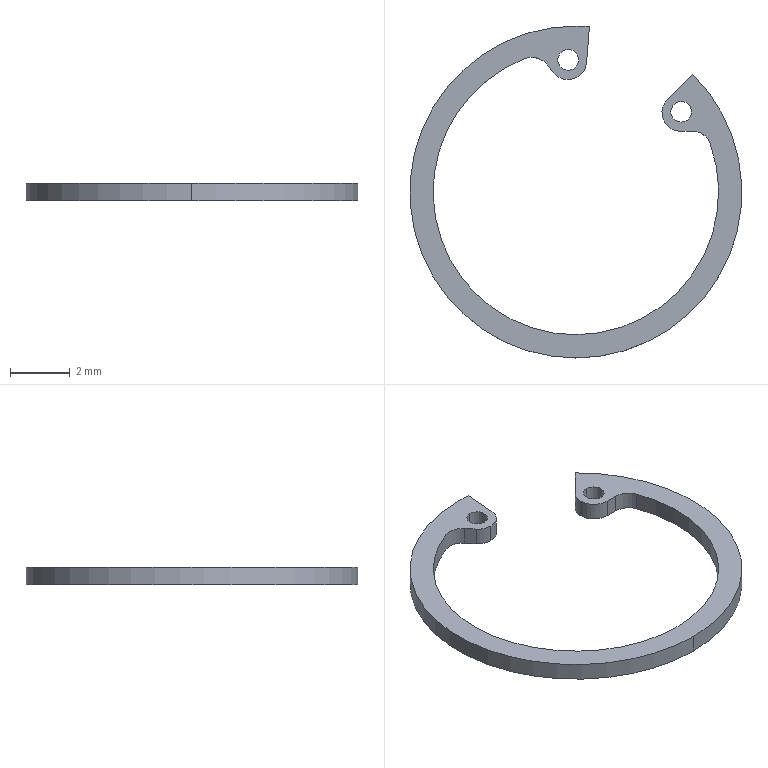Part | SolidWorks | features BaseBody 1 | 1 solid | 21 faces | box 11.1 x 11.1 x 0.6 mm | volume 14.442 mm3 | cylinder 15 | plane 6 | commonest cylinder face diameters 1.243 x6 0.694 x4 11.1 x3 9.546 x2
STEP:
#1=CARTESIAN_POINT('',(558.117,-169.855,283.191));
#2=VERTEX_POINT('',#1);
#3=CARTESIAN_POINT('',(558.117,-169.161,283.191));
#4=VERTEX_POINT('',#3);
#5=CARTESIAN_POINT('',(558.117,-169.508,283.191));
#6=DIRECTION('',(-0.000000001,0.000000003,-1.));
#7=DIRECTION('',(0.,1.,0.000000003));
#8=AXIS2_PLACEMENT_3D('',#5,#6,#7);
#9=CIRCLE('',#8,0.3469);
#10=EDGE_CURVE('',#2,#4,#9,.T.);
#11=ORIENTED_EDGE('',*,*,#10,.F.);
#12=CARTESIAN_POINT('',(558.117,-169.855,282.591));
#13=VERTEX_POINT('',#12);
#14=CARTESIAN_POINT('',(558.117,-169.855,282.591));
#15=DIRECTION('',(-0.000000001,0.000000003,-1.));
#16=VECTOR('',#15,1000.);
#17=LINE('',#14,#16);
#18=EDGE_CURVE('',#2,#13,#17,.T.);
#19=ORIENTED_EDGE('',*,*,#18,.T.);
#20=CARTESIAN_POINT('',(558.117,-169.161,282.591));
#21=VERTEX_POINT('',#20);
#22=CARTESIAN_POINT('',(558.117,-169.508,282.591));
#23=DIRECTION('',(0.000000001,-0.000000003,1.));
#24=DIRECTION('',(0.,1.,0.000000003));
#25=AXIS2_PLACEMENT_3D('',#22,#23,#24);
#26=CIRCLE('',#25,0.3469);
#27=EDGE_CURVE('',#21,#13,#26,.T.);
#28=ORIENTED_EDGE('',*,*,#27,.F.);
#29=CARTESIAN_POINT('',(558.117,-169.161,282.591));
#30=DIRECTION('',(-0.000000001,0.000000003,-1.));
#31=VECTOR('',#30,1000.);
#32=LINE('',#29,#31);
#33=EDGE_CURVE('',#4,#21,#32,.T.);
#34=ORIENTED_EDGE('',*,*,#33,.F.);
#35=EDGE_LOOP('',(#11,#19,#28,#34));
#36=FACE_OUTER_BOUND('',#35,.T.);
#37=CARTESIAN_POINT('',(558.117,-169.508,282.591));
#38=DIRECTION('',(-0.000000001,0.000000003,-1.));
#39=DIRECTION('',(0.,1.,0.000000003));
#40=AXIS2_PLACEMENT_3D('',#37,#38,#39);
#41=CYLINDRICAL_SURFACE('',#40,0.3469);
#42=ADVANCED_FACE('',(#36),#41,.F.);
#43=CARTESIAN_POINT('',(561.892,-171.592,283.191));
#44=VERTEX_POINT('',#43);
#45=CARTESIAN_POINT('',(561.892,-170.898,283.191));
#46=VERTEX_POINT('',#45);
#47=CARTESIAN_POINT('',(561.892,-171.245,283.191));
#48=DIRECTION('',(-0.000000001,0.000000003,-1.));
#49=DIRECTION('',(0.,1.,0.000000003));
#50=AXIS2_PLACEMENT_3D('',#47,#48,#49);
#51=CIRCLE('',#50,0.3469);
#52=EDGE_CURVE('',#44,#46,#51,.T.);
#53=ORIENTED_EDGE('',*,*,#52,.F.);
#54=CARTESIAN_POINT('',(561.892,-171.592,282.591));
#55=VERTEX_POINT('',#54);
#56=CARTESIAN_POINT('',(561.892,-171.592,282.591));
#57=DIRECTION('',(-0.000000001,0.000000003,-1.));
#58=VECTOR('',#57,1000.);
#59=LINE('',#56,#58);
#60=EDGE_CURVE('',#44,#55,#59,.T.);
#61=ORIENTED_EDGE('',*,*,#60,.T.);
#62=CARTESIAN_POINT('',(561.892,-170.898,282.591));
#63=VERTEX_POINT('',#62);
#64=CARTESIAN_POINT('',(561.892,-171.245,282.591));
#65=DIRECTION('',(0.000000001,-0.000000003,1.));
#66=DIRECTION('',(0.,1.,0.000000003));
#67=AXIS2_PLACEMENT_3D('',#64,#65,#66);
#68=CIRCLE('',#67,0.3469);
#69=EDGE_CURVE('',#63,#55,#68,.T.);
#70=ORIENTED_EDGE('',*,*,#69,.F.);
#71=CARTESIAN_POINT('',(561.892,-170.898,282.591));
#72=DIRECTION('',(-0.000000001,0.000000003,-1.));
#73=VECTOR('',#72,1000.);
#74=LINE('',#71,#73);
#75=EDGE_CURVE('',#46,#63,#74,.T.);
#76=ORIENTED_EDGE('',*,*,#75,.F.);
#77=EDGE_LOOP('',(#53,#61,#70,#76));
#78=FACE_OUTER_BOUND('',#77,.T.);
#79=CARTESIAN_POINT('',(561.892,-171.245,282.591));
#80=DIRECTION('',(-0.000000001,0.000000003,-1.));
#81=DIRECTION('',(0.,1.,0.000000003));
#82=AXIS2_PLACEMENT_3D('',#79,#80,#81);
#83=CYLINDRICAL_SURFACE('',#82,0.3469);
#84=ADVANCED_FACE('',(#78),#83,.F.);
#85=CARTESIAN_POINT('',(561.428,-170.838,282.591));
#86=VERTEX_POINT('',#85);
#87=CARTESIAN_POINT('',(561.87,-171.897,282.591));
#88=VERTEX_POINT('',#87);
#89=CARTESIAN_POINT('',(561.87,-171.275,282.591));
#90=DIRECTION('',(0.000000001,-0.000000003,1.));
#91=DIRECTION('',(0.,-1.,-0.000000003));
#92=AXIS2_PLACEMENT_3D('',#89,#90,#91);
#93=CIRCLE('',#92,0.6216);
#94=EDGE_CURVE('',#86,#88,#93,.T.);
#95=ORIENTED_EDGE('',*,*,#94,.T.);
#96=CARTESIAN_POINT('',(561.87,-171.897,283.191));
#97=VERTEX_POINT('',#96);
#98=CARTESIAN_POINT('',(561.87,-171.897,282.591));
#99=DIRECTION('',(0.000000001,-0.000000003,1.));
#100=VECTOR('',#99,1000.);
#101=LINE('',#98,#100);
#102=EDGE_CURVE('',#88,#97,#101,.T.);
#103=ORIENTED_EDGE('',*,*,#102,.T.);
#104=CARTESIAN_POINT('',(561.428,-170.838,283.191));
#105=VERTEX_POINT('',#104);
#106=CARTESIAN_POINT('',(561.87,-171.275,283.191));
#107=DIRECTION('',(0.000000001,-0.000000003,1.));
#108=DIRECTION('',(0.,-1.,-0.000000003));
#109=AXIS2_PLACEMENT_3D('',#106,#107,#108);
#110=CIRCLE('',#109,0.6216);
#111=EDGE_CURVE('',#105,#97,#110,.T.);
#112=ORIENTED_EDGE('',*,*,#111,.F.);
#113=CARTESIAN_POINT('',(561.428,-170.838,282.591));
#114=DIRECTION('',(-0.000000001,0.000000003,-1.));
#115=VECTOR('',#114,1000.);
#116=LINE('',#113,#115);
#117=EDGE_CURVE('',#105,#86,#116,.T.);
#118=ORIENTED_EDGE('',*,*,#117,.T.);
#119=EDGE_LOOP('',(#95,#103,#112,#118));
#120=FACE_OUTER_BOUND('',#119,.T.);
#121=CARTESIAN_POINT('',(561.87,-171.275,282.591));
#122=DIRECTION('',(0.000000001,-0.000000003,1.));
#123=DIRECTION('',(0.,-1.,-0.000000003));
#124=AXIS2_PLACEMENT_3D('',#121,#122,#123);
#125=CYLINDRICAL_SURFACE('',#124,0.6216);
#126=ADVANCED_FACE('',(#120),#125,.T.);
#127=CARTESIAN_POINT('',(558.826,-168.395,282.591));
#128=VERTEX_POINT('',#127);
#129=CARTESIAN_POINT('',(558.371,-168.377,282.591));
#130=VERTEX_POINT('',#129);
#131=CARTESIAN_POINT('',(558.371,-173.927,282.591));
#132=DIRECTION('',(0.000000001,-0.000000003,1.));
#133=DIRECTION('',(0.,-1.,-0.000000003));
#134=AXIS2_PLACEMENT_3D('',#131,#132,#133);
#135=CIRCLE('',#134,5.55);
#136=EDGE_CURVE('',#128,#130,#135,.T.);
#137=ORIENTED_EDGE('',*,*,#136,.T.);
#138=CARTESIAN_POINT('',(558.371,-168.377,283.191));
#139=VERTEX_POINT('',#138);
#140=CARTESIAN_POINT('',(558.371,-168.377,282.591));
#141=DIRECTION('',(0.000000001,-0.000000003,1.));
#142=VECTOR('',#141,1000.);
#143=LINE('',#140,#142);
#144=EDGE_CURVE('',#130,#139,#143,.T.);
#145=ORIENTED_EDGE('',*,*,#144,.T.);
#146=CARTESIAN_POINT('',(558.826,-168.395,283.191));
#147=VERTEX_POINT('',#146);
#148=CARTESIAN_POINT('',(558.371,-173.927,283.191));
#149=DIRECTION('',(0.000000001,-0.000000003,1.));
#150=DIRECTION('',(0.,-1.,-0.000000003));
#151=AXIS2_PLACEMENT_3D('',#148,#149,#150);
#152=CIRCLE('',#151,5.55);
#153=EDGE_CURVE('',#147,#139,#152,.T.);
#154=ORIENTED_EDGE('',*,*,#153,.F.);
#155=CARTESIAN_POINT('',(558.826,-168.395,282.591));
#156=DIRECTION('',(-0.000000001,0.000000003,-1.));
#157=VECTOR('',#156,1000.);
#158=LINE('',#155,#157);
#159=EDGE_CURVE('',#147,#128,#158,.T.);
#160=ORIENTED_EDGE('',*,*,#159,.T.);
#161=EDGE_LOOP('',(#137,#145,#154,#160));
#162=FACE_OUTER_BOUND('',#161,.T.);
#163=CARTESIAN_POINT('',(558.371,-173.927,282.591));
#164=DIRECTION('',(0.000000001,-0.000000003,1.));
#165=DIRECTION('',(0.,-1.,-0.000000003));
#166=AXIS2_PLACEMENT_3D('',#163,#164,#165);
#167=CYLINDRICAL_SURFACE('',#166,5.55);
#168=ADVANCED_FACE('',(#162),#167,.T.);
#169=ORIENTED_EDGE('',*,*,#144,.F.);
#170=CARTESIAN_POINT('',(558.371,-179.477,282.591));
#171=VERTEX_POINT('',#170);
#172=CARTESIAN_POINT('',(558.371,-173.927,282.591));
#173=DIRECTION('',(0.000000001,-0.000000003,1.));
#174=DIRECTION('',(0.,-1.,-0.000000003));
#175=AXIS2_PLACEMENT_3D('',#172,#173,#174);
#176=CIRCLE('',#175,5.55);
#177=EDGE_CURVE('',#130,#171,#176,.T.);
#178=ORIENTED_EDGE('',*,*,#177,.T.);
#179=CARTESIAN_POINT('',(558.371,-179.477,283.191));
#180=VERTEX_POINT('',#179);
#181=CARTESIAN_POINT('',(558.371,-179.477,282.591));
#182=DIRECTION('',(0.000000001,-0.000000003,1.));
#183=VECTOR('',#182,1000.);
#184=LINE('',#181,#183);
#185=EDGE_CURVE('',#171,#180,#184,.T.);
#186=ORIENTED_EDGE('',*,*,#185,.T.);
#187=CARTESIAN_POINT('',(558.371,-173.927,283.191));
#188=DIRECTION('',(0.000000001,-0.000000003,1.));
#189=DIRECTION('',(0.,-1.,-0.000000003));
#190=AXIS2_PLACEMENT_3D('',#187,#188,#189);
#191=CIRCLE('',#190,5.55);
#192=EDGE_CURVE('',#139,#180,#191,.T.);
#193=ORIENTED_EDGE('',*,*,#192,.F.);
#194=EDGE_LOOP('',(#169,#178,#186,#193));
#195=FACE_OUTER_BOUND('',#194,.T.);
#196=CARTESIAN_POINT('',(558.371,-173.927,282.591));
#197=DIRECTION('',(0.000000001,-0.000000003,1.));
#198=DIRECTION('',(0.,-1.,-0.000000003));
#199=AXIS2_PLACEMENT_3D('',#196,#197,#198);
#200=CYLINDRICAL_SURFACE('',#199,5.55);
#201=ADVANCED_FACE('',(#195),#200,.T.);
#202=CARTESIAN_POINT('',(557.631,-169.943,282.591));
#203=VERTEX_POINT('',#202);
#204=CARTESIAN_POINT('',(558.108,-170.166,282.591));
#205=VERTEX_POINT('',#204);
#206=CARTESIAN_POINT('',(558.108,-169.545,282.591));
#207=DIRECTION('',(0.000000001,-0.000000003,1.));
#208=DIRECTION('',(0.,-1.,-0.000000003));
#209=AXIS2_PLACEMENT_3D('',#206,#207,#208);
#210=CIRCLE('',#209,0.6216);
#211=EDGE_CURVE('',#203,#205,#210,.T.);
#212=ORIENTED_EDGE('',*,*,#211,.T.);
#213=CARTESIAN_POINT('',(558.108,-170.166,283.191));
#214=VERTEX_POINT('',#213);
#215=CARTESIAN_POINT('',(558.108,-170.166,282.591));
#216=DIRECTION('',(0.000000001,-0.000000003,1.));
#217=VECTOR('',#216,1000.);
#218=LINE('',#215,#217);
#219=EDGE_CURVE('',#205,#214,#218,.T.);
#220=ORIENTED_EDGE('',*,*,#219,.T.);
#221=CARTESIAN_POINT('',(557.631,-169.943,283.191));
#222=VERTEX_POINT('',#221);
#223=CARTESIAN_POINT('',(558.108,-169.545,283.191));
#224=DIRECTION('',(0.000000001,-0.000000003,1.));
#225=DIRECTION('',(0.,-1.,-0.000000003));
#226=AXIS2_PLACEMENT_3D('',#223,#224,#225);
#227=CIRCLE('',#226,0.6216);
#228=EDGE_CURVE('',#222,#214,#227,.T.);
#229=ORIENTED_EDGE('',*,*,#228,.F.);
#230=CARTESIAN_POINT('',(557.631,-169.943,282.591));
#231=DIRECTION('',(-0.000000001,0.000000003,-1.));
#232=VECTOR('',#231,1000.);
#233=LINE('',#230,#232);
#234=EDGE_CURVE('',#222,#203,#233,.T.);
#235=ORIENTED_EDGE('',*,*,#234,.T.);
#236=EDGE_LOOP('',(#212,#220,#229,#235));
#237=FACE_OUTER_BOUND('',#236,.T.);
#238=CARTESIAN_POINT('',(558.108,-169.545,282.591));
#239=DIRECTION('',(0.000000001,-0.000000003,1.));
#240=DIRECTION('',(0.,-1.,-0.000000003));
#241=AXIS2_PLACEMENT_3D('',#238,#239,#240);
#242=CYLINDRICAL_SURFACE('',#241,0.6216);
#243=ADVANCED_FACE('',(#237),#242,.T.);
#244=CARTESIAN_POINT('',(558.371,-178.7,282.591));
#245=VERTEX_POINT('',#244);
#246=CARTESIAN_POINT('',(562.859,-172.302,282.591));
#247=VERTEX_POINT('',#246);
#248=CARTESIAN_POINT('',(558.371,-173.927,282.591));
#249=DIRECTION('',(0.000000001,-0.000000003,1.));
#250=DIRECTION('',(0.,-1.,-0.000000003));
#251=AXIS2_PLACEMENT_3D('',#248,#249,#250);
#252=CIRCLE('',#251,4.773);
#253=EDGE_CURVE('',#245,#247,#252,.T.);
#254=ORIENTED_EDGE('',*,*,#253,.F.);
#255=CARTESIAN_POINT('',(558.371,-178.7,283.191));
#256=VERTEX_POINT('',#255);
#257=CARTESIAN_POINT('',(558.371,-178.7,282.591));
#258=DIRECTION('',(0.000000001,-0.000000003,1.));
#259=VECTOR('',#258,1000.);
#260=LINE('',#257,#259);
#261=EDGE_CURVE('',#245,#256,#260,.T.);
#262=ORIENTED_EDGE('',*,*,#261,.T.);
#263=CARTESIAN_POINT('',(562.859,-172.302,283.191));
#264=VERTEX_POINT('',#263);
#265=CARTESIAN_POINT('',(558.371,-173.927,283.191));
#266=DIRECTION('',(-0.000000001,0.000000003,-1.));
#267=DIRECTION('',(0.,-1.,-0.000000003));
#268=AXIS2_PLACEMENT_3D('',#265,#266,#267);
#269=CIRCLE('',#268,4.773);
#270=EDGE_CURVE('',#264,#256,#269,.T.);
#271=ORIENTED_EDGE('',*,*,#270,.F.);
#272=CARTESIAN_POINT('',(562.859,-172.302,282.591));
#273=DIRECTION('',(0.000000001,-0.000000003,1.));
#274=VECTOR('',#273,1000.);
#275=LINE('',#272,#274);
#276=EDGE_CURVE('',#247,#264,#275,.T.);
#277=ORIENTED_EDGE('',*,*,#276,.F.);
#278=EDGE_LOOP('',(#254,#262,#271,#277));
#279=FACE_OUTER_BOUND('',#278,.T.);
#280=CARTESIAN_POINT('',(558.371,-173.927,282.591));
#281=DIRECTION('',(0.000000001,-0.000000003,1.));
#282=DIRECTION('',(0.,-1.,-0.000000003));
#283=AXIS2_PLACEMENT_3D('',#280,#281,#282);
#284=CYLINDRICAL_SURFACE('',#283,4.773);
#285=ADVANCED_FACE('',(#279),#284,.F.);
#286=CARTESIAN_POINT('',(558.117,-169.508,283.191));
#287=DIRECTION('',(-0.000000001,0.000000003,-1.));
#288=DIRECTION('',(0.,1.,0.000000003));
#289=AXIS2_PLACEMENT_3D('',#286,#287,#288);
#290=CIRCLE('',#289,0.3469);
#291=EDGE_CURVE('',#4,#2,#290,.T.);
#292=ORIENTED_EDGE('',*,*,#291,.T.);
#293=ORIENTED_EDGE('',*,*,#10,.T.);
#294=EDGE_LOOP('',(#292,#293));
#295=FACE_BOUND('',#294,.T.);
#296=CARTESIAN_POINT('',(561.892,-171.245,283.191));
#297=DIRECTION('',(-0.000000001,0.000000003,-1.));
#298=DIRECTION('',(0.,1.,0.000000003));
#299=AXIS2_PLACEMENT_3D('',#296,#297,#298);
#300=CIRCLE('',#299,0.3469);
#301=EDGE_CURVE('',#46,#44,#300,.T.);
#302=ORIENTED_EDGE('',*,*,#301,.T.);
#303=ORIENTED_EDGE('',*,*,#52,.T.);
#304=EDGE_LOOP('',(#302,#303));
#305=FACE_BOUND('',#304,.T.);
#306=CARTESIAN_POINT('',(562.275,-169.982,283.191));
#307=VERTEX_POINT('',#306);
#308=CARTESIAN_POINT('',(562.275,-169.982,283.191));
#309=DIRECTION('',(-0.7035,-0.7107,-0.000000002));
#310=VECTOR('',#309,1000.);
#311=LINE('',#308,#310);
#312=EDGE_CURVE('',#307,#105,#311,.T.);
#313=ORIENTED_EDGE('',*,*,#312,.T.);
#314=ORIENTED_EDGE('',*,*,#111,.T.);
#315=CARTESIAN_POINT('',(561.877,-171.897,283.191));
#316=VERTEX_POINT('',#315);
#317=CARTESIAN_POINT('',(561.87,-171.275,283.191));
#318=DIRECTION('',(0.000000001,-0.000000003,1.));
#319=DIRECTION('',(0.,-1.,-0.000000003));
#320=AXIS2_PLACEMENT_3D('',#317,#318,#319);
#321=CIRCLE('',#320,0.6216);
#322=EDGE_CURVE('',#97,#316,#321,.T.);
#323=ORIENTED_EDGE('',*,*,#322,.T.);
#324=CARTESIAN_POINT('',(562.267,-171.892,283.191));
#325=VERTEX_POINT('',#324);
#326=CARTESIAN_POINT('',(561.877,-171.897,283.191));
#327=DIRECTION('',(0.9999,0.01191,-0.000000001));
#328=VECTOR('',#327,1000.);
#329=LINE('',#326,#328);
#330=EDGE_CURVE('',#316,#325,#329,.T.);
#331=ORIENTED_EDGE('',*,*,#330,.T.);
#332=CARTESIAN_POINT('',(562.275,-172.514,283.191));
#333=DIRECTION('',(-0.000000001,0.000000003,-1.));
#334=DIRECTION('',(0.,-1.,-0.000000003));
#335=AXIS2_PLACEMENT_3D('',#332,#333,#334);
#336=CIRCLE('',#335,0.6216);
#337=EDGE_CURVE('',#325,#264,#336,.T.);
#338=ORIENTED_EDGE('',*,*,#337,.T.);
#339=ORIENTED_EDGE('',*,*,#270,.T.);
#340=CARTESIAN_POINT('',(556.684,-169.461,283.191));
#341=VERTEX_POINT('',#340);
#342=CARTESIAN_POINT('',(558.371,-173.927,283.191));
#343=DIRECTION('',(-0.000000001,0.000000003,-1.));
#344=DIRECTION('',(0.,-1.,-0.000000003));
#345=AXIS2_PLACEMENT_3D('',#342,#343,#344);
#346=CIRCLE('',#345,4.773);
#347=EDGE_CURVE('',#256,#341,#346,.T.);
#348=ORIENTED_EDGE('',*,*,#347,.T.);
#349=CARTESIAN_POINT('',(557.381,-169.644,283.191));
#350=VERTEX_POINT('',#349);
#351=CARTESIAN_POINT('',(556.904,-170.043,283.191));
#352=DIRECTION('',(-0.000000001,0.000000003,-1.));
#353=DIRECTION('',(0.,-1.,-0.000000003));
#354=AXIS2_PLACEMENT_3D('',#351,#352,#353);
#355=CIRCLE('',#354,0.6216);
#356=EDGE_CURVE('',#341,#350,#355,.T.);
#357=ORIENTED_EDGE('',*,*,#356,.T.);
#358=CARTESIAN_POINT('',(557.381,-169.644,283.191));
#359=DIRECTION('',(0.6416,-0.7671,-0.000000003));
#360=VECTOR('',#359,1000.);
#361=LINE('',#358,#360);
#362=EDGE_CURVE('',#350,#222,#361,.T.);
#363=ORIENTED_EDGE('',*,*,#362,.T.);
#364=ORIENTED_EDGE('',*,*,#228,.T.);
#365=CARTESIAN_POINT('',(558.727,-169.596,283.191));
#366=VERTEX_POINT('',#365);
#367=CARTESIAN_POINT('',(558.108,-169.545,283.191));
#368=DIRECTION('',(0.000000001,-0.000000003,1.));
#369=DIRECTION('',(0.,-1.,-0.000000003));
#370=AXIS2_PLACEMENT_3D('',#367,#368,#369);
#371=CIRCLE('',#370,0.6216);
#372=EDGE_CURVE('',#214,#366,#371,.T.);
#373=ORIENTED_EDGE('',*,*,#372,.T.);
#374=CARTESIAN_POINT('',(558.727,-169.596,283.191));
#375=DIRECTION('',(0.08202,0.9966,0.000000003));
#376=VECTOR('',#375,1000.);
#377=LINE('',#374,#376);
#378=EDGE_CURVE('',#366,#147,#377,.T.);
#379=ORIENTED_EDGE('',*,*,#378,.T.);
#380=ORIENTED_EDGE('',*,*,#153,.T.);
#381=ORIENTED_EDGE('',*,*,#192,.T.);
#382=CARTESIAN_POINT('',(558.371,-173.927,283.191));
#383=DIRECTION('',(0.000000001,-0.000000003,1.));
#384=DIRECTION('',(0.,-1.,-0.000000003));
#385=AXIS2_PLACEMENT_3D('',#382,#383,#384);
#386=CIRCLE('',#385,5.55);
#387=EDGE_CURVE('',#180,#307,#386,.T.);
#388=ORIENTED_EDGE('',*,*,#387,.T.);
#389=EDGE_LOOP('',(#313,#314,#323,#331,#338,#339,#348,#357,#363,#364,#373,#379,#380,#381,#388));
#390=FACE_OUTER_BOUND('',#389,.T.);
#391=CARTESIAN_POINT('',(558.5,-173.641,283.191));
#392=DIRECTION('',(0.000000001,-0.000000003,1.));
#393=DIRECTION('',(0.,-1.,-0.000000003));
#394=AXIS2_PLACEMENT_3D('',#391,#392,#393);
#395=PLANE('',#394);
#396=ADVANCED_FACE('',(#295,#305,#390),#395,.T.);
#397=ORIENTED_EDGE('',*,*,#18,.F.);
#398=ORIENTED_EDGE('',*,*,#291,.F.);
#399=ORIENTED_EDGE('',*,*,#33,.T.);
#400=CARTESIAN_POINT('',(558.117,-169.508,282.591));
#401=DIRECTION('',(0.000000001,-0.000000003,1.));
#402=DIRECTION('',(0.,1.,0.000000003));
#403=AXIS2_PLACEMENT_3D('',#400,#401,#402);
#404=CIRCLE('',#403,0.3469);
#405=EDGE_CURVE('',#13,#21,#404,.T.);
#406=ORIENTED_EDGE('',*,*,#405,.F.);
#407=EDGE_LOOP('',(#397,#398,#399,#406));
#408=FACE_OUTER_BOUND('',#407,.T.);
#409=CARTESIAN_POINT('',(558.117,-169.508,282.591));
#410=DIRECTION('',(-0.000000001,0.000000003,-1.));
#411=DIRECTION('',(0.,1.,0.000000003));
#412=AXIS2_PLACEMENT_3D('',#409,#410,#411);
#413=CYLINDRICAL_SURFACE('',#412,0.3469);
#414=ADVANCED_FACE('',(#408),#413,.F.);
#415=ORIENTED_EDGE('',*,*,#60,.F.);
#416=ORIENTED_EDGE('',*,*,#301,.F.);
#417=ORIENTED_EDGE('',*,*,#75,.T.);
#418=CARTESIAN_POINT('',(561.892,-171.245,282.591));
#419=DIRECTION('',(0.000000001,-0.000000003,1.));
#420=DIRECTION('',(0.,1.,0.000000003));
#421=AXIS2_PLACEMENT_3D('',#418,#419,#420);
#422=CIRCLE('',#421,0.3469);
#423=EDGE_CURVE('',#55,#63,#422,.T.);
#424=ORIENTED_EDGE('',*,*,#423,.F.);
#425=EDGE_LOOP('',(#415,#416,#417,#424));
#426=FACE_OUTER_BOUND('',#425,.T.);
#427=CARTESIAN_POINT('',(561.892,-171.245,282.591));
#428=DIRECTION('',(-0.000000001,0.000000003,-1.));
#429=DIRECTION('',(0.,1.,0.000000003));
#430=AXIS2_PLACEMENT_3D('',#427,#428,#429);
#431=CYLINDRICAL_SURFACE('',#430,0.3469);
#432=ADVANCED_FACE('',(#426),#431,.F.);
#433=ORIENTED_EDGE('',*,*,#102,.F.);
#434=CARTESIAN_POINT('',(561.877,-171.897,282.591));
#435=VERTEX_POINT('',#434);
#436=CARTESIAN_POINT('',(561.87,-171.275,282.591));
#437=DIRECTION('',(0.000000001,-0.000000003,1.));
#438=DIRECTION('',(0.,-1.,-0.000000003));
#439=AXIS2_PLACEMENT_3D('',#436,#437,#438);
#440=CIRCLE('',#439,0.6216);
#441=EDGE_CURVE('',#88,#435,#440,.T.);
#442=ORIENTED_EDGE('',*,*,#441,.T.);
#443=CARTESIAN_POINT('',(561.877,-171.897,282.591));
#444=DIRECTION('',(0.,0.000000003,-1.));
#445=VECTOR('',#444,1000.);
#446=LINE('',#443,#445);
#447=EDGE_CURVE('',#316,#435,#446,.T.);
#448=ORIENTED_EDGE('',*,*,#447,.F.);
#449=ORIENTED_EDGE('',*,*,#322,.F.);
#450=EDGE_LOOP('',(#433,#442,#448,#449));
#451=FACE_OUTER_BOUND('',#450,.T.);
#452=CARTESIAN_POINT('',(561.87,-171.275,282.591));
#453=DIRECTION('',(0.000000001,-0.000000003,1.));
#454=DIRECTION('',(0.,-1.,-0.000000003));
#455=AXIS2_PLACEMENT_3D('',#452,#453,#454);
#456=CYLINDRICAL_SURFACE('',#455,0.6216);
#457=ADVANCED_FACE('',(#451),#456,.T.);
#458=CARTESIAN_POINT('',(562.275,-169.982,282.591));
#459=VERTEX_POINT('',#458);
#460=CARTESIAN_POINT('',(561.428,-170.838,282.591));
#461=DIRECTION('',(-0.7035,-0.7107,0.));
#462=VECTOR('',#461,1000.);
#463=LINE('',#460,#462);
#464=EDGE_CURVE('',#459,#86,#463,.T.);
#465=ORIENTED_EDGE('',*,*,#464,.T.);
#466=ORIENTED_EDGE('',*,*,#117,.F.);
#467=ORIENTED_EDGE('',*,*,#312,.F.);
#468=CARTESIAN_POINT('',(562.275,-169.982,282.591));
#469=DIRECTION('',(-0.000000002,0.000000002,-1.));
#470=VECTOR('',#469,1000.);
#471=LINE('',#468,#470);
#472=EDGE_CURVE('',#307,#459,#471,.T.);
#473=ORIENTED_EDGE('',*,*,#472,.T.);
#474=EDGE_LOOP('',(#465,#466,#467,#473));
#475=FACE_OUTER_BOUND('',#474,.T.);
#476=CARTESIAN_POINT('',(561.428,-170.838,282.591));
#477=DIRECTION('',(-0.7107,0.7035,0.000000003));
#478=DIRECTION('',(-0.7035,-0.7107,0.));
#479=AXIS2_PLACEMENT_3D('',#476,#477,#478);
#480=PLANE('',#479);
#481=ADVANCED_FACE('',(#475),#480,.T.);
#482=ORIENTED_EDGE('',*,*,#185,.F.);
#483=CARTESIAN_POINT('',(558.371,-173.927,282.591));
#484=DIRECTION('',(0.000000001,-0.000000003,1.));
#485=DIRECTION('',(0.,-1.,-0.000000003));
#486=AXIS2_PLACEMENT_3D('',#483,#484,#485);
#487=CIRCLE('',#486,5.55);
#488=EDGE_CURVE('',#171,#459,#487,.T.);
#489=ORIENTED_EDGE('',*,*,#488,.T.);
#490=ORIENTED_EDGE('',*,*,#472,.F.);
#491=ORIENTED_EDGE('',*,*,#387,.F.);
#492=EDGE_LOOP('',(#482,#489,#490,#491));
#493=FACE_OUTER_BOUND('',#492,.T.);
#494=CARTESIAN_POINT('',(558.371,-173.927,282.591));
#495=DIRECTION('',(0.000000001,-0.000000003,1.));
#496=DIRECTION('',(0.,-1.,-0.000000003));
#497=AXIS2_PLACEMENT_3D('',#494,#495,#496);
#498=CYLINDRICAL_SURFACE('',#497,5.55);
#499=ADVANCED_FACE('',(#493),#498,.T.);
#500=CARTESIAN_POINT('',(558.727,-169.596,282.591));
#501=VERTEX_POINT('',#500);
#502=CARTESIAN_POINT('',(558.826,-168.395,282.591));
#503=DIRECTION('',(0.08202,0.9966,0.));
#504=VECTOR('',#503,1000.);
#505=LINE('',#502,#504);
#506=EDGE_CURVE('',#501,#128,#505,.T.);
#507=ORIENTED_EDGE('',*,*,#506,.T.);
#508=ORIENTED_EDGE('',*,*,#159,.F.);
#509=ORIENTED_EDGE('',*,*,#378,.F.);
#510=CARTESIAN_POINT('',(558.727,-169.596,282.591));
#511=DIRECTION('',(-0.000000001,0.,-1.));
#512=VECTOR('',#511,1000.);
#513=LINE('',#510,#512);
#514=EDGE_CURVE('',#366,#501,#513,.T.);
#515=ORIENTED_EDGE('',*,*,#514,.T.);
#516=EDGE_LOOP('',(#507,#508,#509,#515));
#517=FACE_OUTER_BOUND('',#516,.T.);
#518=CARTESIAN_POINT('',(558.826,-168.395,282.591));
#519=DIRECTION('',(0.9966,-0.08202,-0.000000001));
#520=DIRECTION('',(0.08202,0.9966,0.));
#521=AXIS2_PLACEMENT_3D('',#518,#519,#520);
#522=PLANE('',#521);
#523=ADVANCED_FACE('',(#517),#522,.T.);
#524=ORIENTED_EDGE('',*,*,#219,.F.);
#525=CARTESIAN_POINT('',(558.108,-169.545,282.591));
#526=DIRECTION('',(0.000000001,-0.000000003,1.));
#527=DIRECTION('',(0.,-1.,-0.000000003));
#528=AXIS2_PLACEMENT_3D('',#525,#526,#527);
#529=CIRCLE('',#528,0.6216);
#530=EDGE_CURVE('',#205,#501,#529,.T.);
#531=ORIENTED_EDGE('',*,*,#530,.T.);
#532=ORIENTED_EDGE('',*,*,#514,.F.);
#533=ORIENTED_EDGE('',*,*,#372,.F.);
#534=EDGE_LOOP('',(#524,#531,#532,#533));
#535=FACE_OUTER_BOUND('',#534,.T.);
#536=CARTESIAN_POINT('',(558.108,-169.545,282.591));
#537=DIRECTION('',(0.000000001,-0.000000003,1.));
#538=DIRECTION('',(0.,-1.,-0.000000003));
#539=AXIS2_PLACEMENT_3D('',#536,#537,#538);
#540=CYLINDRICAL_SURFACE('',#539,0.6216);
#541=ADVANCED_FACE('',(#535),#540,.T.);
#542=CARTESIAN_POINT('',(557.381,-169.644,282.591));
#543=VERTEX_POINT('',#542);
#544=CARTESIAN_POINT('',(557.631,-169.943,282.591));
#545=DIRECTION('',(0.6416,-0.7671,0.));
#546=VECTOR('',#545,1000.);
#547=LINE('',#544,#546);
#548=EDGE_CURVE('',#543,#203,#547,.T.);
#549=ORIENTED_EDGE('',*,*,#548,.T.);
#550=ORIENTED_EDGE('',*,*,#234,.F.);
#551=ORIENTED_EDGE('',*,*,#362,.F.);
#552=CARTESIAN_POINT('',(557.381,-169.644,282.591));
#553=DIRECTION('',(0.000000001,0.000000001,-1.));
#554=VECTOR('',#553,1000.);
#555=LINE('',#552,#554);
#556=EDGE_CURVE('',#350,#543,#555,.T.);
#557=ORIENTED_EDGE('',*,*,#556,.T.);
#558=EDGE_LOOP('',(#549,#550,#551,#557));
#559=FACE_OUTER_BOUND('',#558,.T.);
#560=CARTESIAN_POINT('',(557.631,-169.943,282.591));
#561=DIRECTION('',(-0.7671,-0.6416,-0.000000002));
#562=DIRECTION('',(0.6416,-0.7671,0.));
#563=AXIS2_PLACEMENT_3D('',#560,#561,#562);
#564=PLANE('',#563);
#565=ADVANCED_FACE('',(#559),#564,.T.);
#566=CARTESIAN_POINT('',(556.684,-169.461,282.591));
#567=VERTEX_POINT('',#566);
#568=CARTESIAN_POINT('',(556.684,-169.461,282.591));
#569=DIRECTION('',(0.000000001,-0.000000003,1.));
#570=VECTOR('',#569,1000.);
#571=LINE('',#568,#570);
#572=EDGE_CURVE('',#567,#341,#571,.T.);
#573=ORIENTED_EDGE('',*,*,#572,.F.);
#574=CARTESIAN_POINT('',(556.904,-170.043,282.591));
#575=DIRECTION('',(0.000000001,-0.000000003,1.));
#576=DIRECTION('',(0.,-1.,-0.000000003));
#577=AXIS2_PLACEMENT_3D('',#574,#575,#576);
#578=CIRCLE('',#577,0.6216);
#579=EDGE_CURVE('',#543,#567,#578,.T.);
#580=ORIENTED_EDGE('',*,*,#579,.F.);
#581=ORIENTED_EDGE('',*,*,#556,.F.);
#582=ORIENTED_EDGE('',*,*,#356,.F.);
#583=EDGE_LOOP('',(#573,#580,#581,#582));
#584=FACE_OUTER_BOUND('',#583,.T.);
#585=CARTESIAN_POINT('',(556.904,-170.043,282.591));
#586=DIRECTION('',(0.000000001,-0.000000003,1.));
#587=DIRECTION('',(0.,-1.,-0.000000003));
#588=AXIS2_PLACEMENT_3D('',#585,#586,#587);
#589=CYLINDRICAL_SURFACE('',#588,0.6216);
#590=ADVANCED_FACE('',(#584),#589,.F.);
#591=ORIENTED_EDGE('',*,*,#261,.F.);
#592=CARTESIAN_POINT('',(558.371,-173.927,282.591));
#593=DIRECTION('',(0.000000001,-0.000000003,1.));
#594=DIRECTION('',(0.,-1.,-0.000000003));
#595=AXIS2_PLACEMENT_3D('',#592,#593,#594);
#596=CIRCLE('',#595,4.773);
#597=EDGE_CURVE('',#567,#245,#596,.T.);
#598=ORIENTED_EDGE('',*,*,#597,.F.);
#599=ORIENTED_EDGE('',*,*,#572,.T.);
#600=ORIENTED_EDGE('',*,*,#347,.F.);
#601=EDGE_LOOP('',(#591,#598,#599,#600));
#602=FACE_OUTER_BOUND('',#601,.T.);
#603=CARTESIAN_POINT('',(558.371,-173.927,282.591));
#604=DIRECTION('',(0.000000001,-0.000000003,1.));
#605=DIRECTION('',(0.,-1.,-0.000000003));
#606=AXIS2_PLACEMENT_3D('',#603,#604,#605);
#607=CYLINDRICAL_SURFACE('',#606,4.773);
#608=ADVANCED_FACE('',(#602),#607,.F.);
#609=CARTESIAN_POINT('',(562.267,-171.892,282.591));
#610=VERTEX_POINT('',#609);
#611=CARTESIAN_POINT('',(562.267,-171.892,282.591));
#612=DIRECTION('',(0.000000001,-0.000000003,1.));
#613=VECTOR('',#612,1000.);
#614=LINE('',#611,#613);
#615=EDGE_CURVE('',#610,#325,#614,.T.);
#616=ORIENTED_EDGE('',*,*,#615,.F.);
#617=CARTESIAN_POINT('',(562.275,-172.514,282.591));
#618=DIRECTION('',(0.000000001,-0.000000003,1.));
#619=DIRECTION('',(0.,-1.,-0.000000003));
#620=AXIS2_PLACEMENT_3D('',#617,#618,#619);
#621=CIRCLE('',#620,0.6216);
#622=EDGE_CURVE('',#247,#610,#621,.T.);
#623=ORIENTED_EDGE('',*,*,#622,.F.);
#624=ORIENTED_EDGE('',*,*,#276,.T.);
#625=ORIENTED_EDGE('',*,*,#337,.F.);
#626=EDGE_LOOP('',(#616,#623,#624,#625));
#627=FACE_OUTER_BOUND('',#626,.T.);
#628=CARTESIAN_POINT('',(562.275,-172.514,282.591));
#629=DIRECTION('',(0.000000001,-0.000000003,1.));
#630=DIRECTION('',(0.,-1.,-0.000000003));
#631=AXIS2_PLACEMENT_3D('',#628,#629,#630);
#632=CYLINDRICAL_SURFACE('',#631,0.6216);
#633=ADVANCED_FACE('',(#627),#632,.F.);
#634=CARTESIAN_POINT('',(562.267,-171.892,282.591));
#635=DIRECTION('',(0.9999,0.01191,0.));
#636=VECTOR('',#635,1000.);
#637=LINE('',#634,#636);
#638=EDGE_CURVE('',#435,#610,#637,.T.);
#639=ORIENTED_EDGE('',*,*,#638,.T.);
#640=ORIENTED_EDGE('',*,*,#615,.T.);
#641=ORIENTED_EDGE('',*,*,#330,.F.);
#642=ORIENTED_EDGE('',*,*,#447,.T.);
#643=EDGE_LOOP('',(#639,#640,#641,#642));
#644=FACE_OUTER_BOUND('',#643,.T.);
#645=CARTESIAN_POINT('',(562.267,-171.892,282.591));
#646=DIRECTION('',(0.01191,-0.9999,-0.000000003));
#647=DIRECTION('',(0.9999,0.01191,0.));
#648=AXIS2_PLACEMENT_3D('',#645,#646,#647);
#649=PLANE('',#648);
#650=ADVANCED_FACE('',(#644),#649,.T.);
#651=ORIENTED_EDGE('',*,*,#27,.T.);
#652=ORIENTED_EDGE('',*,*,#405,.T.);
#653=EDGE_LOOP('',(#651,#652));
#654=FACE_BOUND('',#653,.T.);
#655=ORIENTED_EDGE('',*,*,#69,.T.);
#656=ORIENTED_EDGE('',*,*,#423,.T.);
#657=EDGE_LOOP('',(#655,#656));
#658=FACE_BOUND('',#657,.T.);
#659=ORIENTED_EDGE('',*,*,#638,.F.);
#660=ORIENTED_EDGE('',*,*,#441,.F.);
#661=ORIENTED_EDGE('',*,*,#94,.F.);
#662=ORIENTED_EDGE('',*,*,#464,.F.);
#663=ORIENTED_EDGE('',*,*,#488,.F.);
#664=ORIENTED_EDGE('',*,*,#177,.F.);
#665=ORIENTED_EDGE('',*,*,#136,.F.);
#666=ORIENTED_EDGE('',*,*,#506,.F.);
#667=ORIENTED_EDGE('',*,*,#530,.F.);
#668=ORIENTED_EDGE('',*,*,#211,.F.);
#669=ORIENTED_EDGE('',*,*,#548,.F.);
#670=ORIENTED_EDGE('',*,*,#579,.T.);
#671=ORIENTED_EDGE('',*,*,#597,.T.);
#672=ORIENTED_EDGE('',*,*,#253,.T.);
#673=ORIENTED_EDGE('',*,*,#622,.T.);
#674=EDGE_LOOP('',(#659,#660,#661,#662,#663,#664,#665,#666,#667,#668,#669,#670,#671,#672,#673));
#675=FACE_OUTER_BOUND('',#674,.T.);
#676=CARTESIAN_POINT('',(558.5,-173.641,282.591));
#677=DIRECTION('',(0.000000001,-0.000000003,1.));
#678=DIRECTION('',(0.,-1.,-0.000000003));
#679=AXIS2_PLACEMENT_3D('',#676,#677,#678);
#680=PLANE('',#679);
#681=ADVANCED_FACE('',(#654,#658,#675),#680,.F.);
#682=CLOSED_SHELL('',(#42,#84,#126,#168,#201,#243,#285,#396,#414,#432,#457,#481,#499,#523,#541,#565,#590,#608,#633,#650,#681));
#683=MANIFOLD_SOLID_BREP('',#682);
#684=CARTESIAN_POINT('',(0.,0.,0.));
#685=DIRECTION('',(0.,0.,1.));
#686=DIRECTION('',(1.,0.,0.));
#687=AXIS2_PLACEMENT_3D('',#684,#685,#686);
#688=(LENGTH_UNIT()NAMED_UNIT(*)SI_UNIT(.MILLI.,.METRE.));
#689=UNCERTAINTY_MEASURE_WITH_UNIT(LENGTH_MEASURE(0.00001),#688,'','');
#690=(NAMED_UNIT(*)PLANE_ANGLE_UNIT()SI_UNIT($,.RADIAN.));
#691=(NAMED_UNIT(*)SI_UNIT($,.STERADIAN.)SOLID_ANGLE_UNIT());
#692=(GEOMETRIC_REPRESENTATION_CONTEXT(3)GLOBAL_UNCERTAINTY_ASSIGNED_CONTEXT((#689))GLOBAL_UNIT_ASSIGNED_CONTEXT((#688,#690,#691))REPRESENTATION_CONTEXT('',''));
#693=ADVANCED_BREP_SHAPE_REPRESENTATION('',(#683,#687),#692);